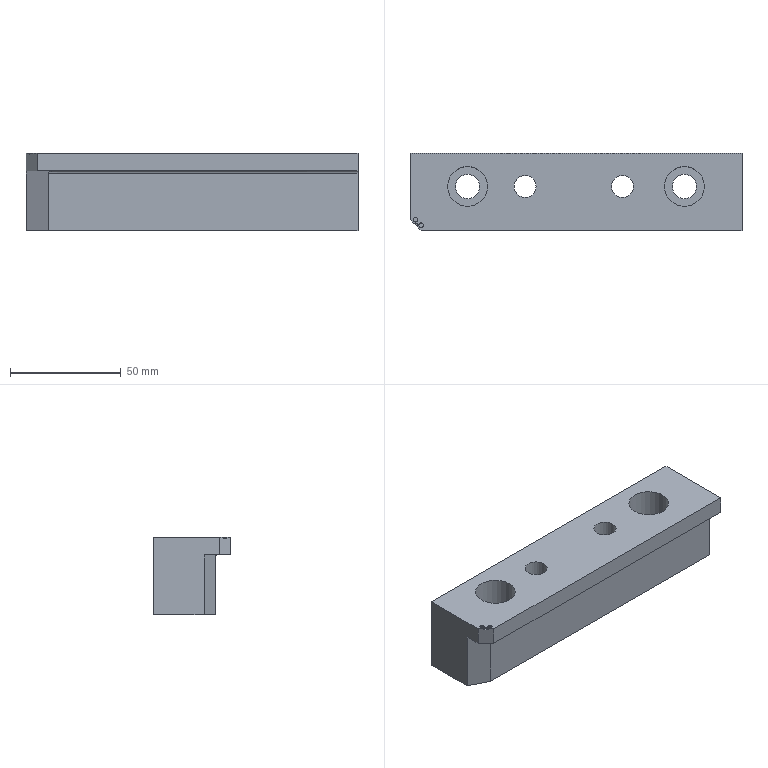Part | NX | features DIE-2 2 | 1 solid | 25 faces | box 150 x 35 x 35 mm | volume 137394 mm3 | plane 15 | cylinder 10 | commonest cylinder face diameters 2 x4 10 x2 11.007 x2 18 x2
STEP:
#1=CARTESIAN_POINT('',(2244.094,-778.422,858.716));
#2=VERTEX_POINT('',#1);
#3=CARTESIAN_POINT('',(2239.094,-778.422,858.716));
#4=DIRECTION('',(0.,0.,1.));
#5=DIRECTION('',(1.,0.,0.));
#6=AXIS2_PLACEMENT_3D('',#3,#4,#5);
#7=CIRCLE('',#6,5.);
#8=EDGE_CURVE('',#2,#2,#7,.T.);
#9=ORIENTED_EDGE('',*,*,#8,.F.);
#10=EDGE_LOOP('',(#9));
#11=FACE_BOUND('',#10,.T.);
#12=CARTESIAN_POINT('',(2244.094,-778.422,893.716));
#13=VERTEX_POINT('',#12);
#14=CARTESIAN_POINT('',(2239.094,-778.422,893.716));
#15=DIRECTION('',(0.,0.,-1.));
#16=DIRECTION('',(1.,0.,0.));
#17=AXIS2_PLACEMENT_3D('',#14,#15,#16);
#18=CIRCLE('',#17,5.);
#19=EDGE_CURVE('',#13,#13,#18,.T.);
#20=ORIENTED_EDGE('',*,*,#19,.F.);
#21=EDGE_LOOP('',(#20));
#22=FACE_BOUND('',#21,.T.);
#23=CARTESIAN_POINT('',(2239.094,-778.422,890.716));
#24=DIRECTION('',(0.,0.,1.));
#25=DIRECTION('',(-1.,0.,0.));
#26=AXIS2_PLACEMENT_3D('',#23,#24,#25);
#27=CYLINDRICAL_SURFACE('',#26,5.);
#28=ADVANCED_FACE('',(#11,#22),#27,.F.);
#29=CARTESIAN_POINT('',(2276.094,-778.422,877.716));
#30=VERTEX_POINT('',#29);
#31=CARTESIAN_POINT('',(2267.094,-778.422,877.716));
#32=DIRECTION('',(0.,0.,-1.));
#33=DIRECTION('',(1.,0.,0.));
#34=AXIS2_PLACEMENT_3D('',#31,#32,#33);
#35=CIRCLE('',#34,9.);
#36=EDGE_CURVE('',#30,#30,#35,.T.);
#37=ORIENTED_EDGE('',*,*,#36,.T.);
#38=EDGE_LOOP('',(#37));
#39=FACE_BOUND('',#38,.T.);
#40=CARTESIAN_POINT('',(2276.094,-778.422,893.716));
#41=VERTEX_POINT('',#40);
#42=CARTESIAN_POINT('',(2267.094,-778.422,893.716));
#43=DIRECTION('',(0.,0.,-1.));
#44=DIRECTION('',(1.,0.,0.));
#45=AXIS2_PLACEMENT_3D('',#42,#43,#44);
#46=CIRCLE('',#45,9.);
#47=EDGE_CURVE('',#41,#41,#46,.T.);
#48=ORIENTED_EDGE('',*,*,#47,.F.);
#49=EDGE_LOOP('',(#48));
#50=FACE_BOUND('',#49,.T.);
#51=CARTESIAN_POINT('',(2267.094,-778.422,884.216));
#52=DIRECTION('',(0.,0.,-1.));
#53=DIRECTION('',(-1.,0.,0.));
#54=AXIS2_PLACEMENT_3D('',#51,#52,#53);
#55=CYLINDRICAL_SURFACE('',#54,9.);
#56=ADVANCED_FACE('',(#39,#50),#55,.F.);
#57=CARTESIAN_POINT('',(2178.094,-778.422,877.716));
#58=VERTEX_POINT('',#57);
#59=CARTESIAN_POINT('',(2169.094,-778.422,877.716));
#60=DIRECTION('',(0.,0.,-1.));
#61=DIRECTION('',(1.,0.,0.));
#62=AXIS2_PLACEMENT_3D('',#59,#60,#61);
#63=CIRCLE('',#62,9.);
#64=EDGE_CURVE('',#58,#58,#63,.T.);
#65=ORIENTED_EDGE('',*,*,#64,.T.);
#66=EDGE_LOOP('',(#65));
#67=FACE_BOUND('',#66,.T.);
#68=CARTESIAN_POINT('',(2178.094,-778.422,893.716));
#69=VERTEX_POINT('',#68);
#70=CARTESIAN_POINT('',(2169.094,-778.422,893.716));
#71=DIRECTION('',(0.,0.,-1.));
#72=DIRECTION('',(1.,0.,0.));
#73=AXIS2_PLACEMENT_3D('',#70,#71,#72);
#74=CIRCLE('',#73,9.);
#75=EDGE_CURVE('',#69,#69,#74,.T.);
#76=ORIENTED_EDGE('',*,*,#75,.F.);
#77=EDGE_LOOP('',(#76));
#78=FACE_BOUND('',#77,.T.);
#79=CARTESIAN_POINT('',(2169.094,-778.422,884.216));
#80=DIRECTION('',(0.,0.,-1.));
#81=DIRECTION('',(-1.,0.,0.));
#82=AXIS2_PLACEMENT_3D('',#79,#80,#81);
#83=CYLINDRICAL_SURFACE('',#82,9.);
#84=ADVANCED_FACE('',(#67,#78),#83,.F.);
#85=CARTESIAN_POINT('',(2200.094,-778.422,858.716));
#86=VERTEX_POINT('',#85);
#87=CARTESIAN_POINT('',(2195.094,-778.422,858.716));
#88=DIRECTION('',(0.,0.,-1.));
#89=DIRECTION('',(1.,0.,0.));
#90=AXIS2_PLACEMENT_3D('',#87,#88,#89);
#91=CIRCLE('',#90,5.);
#92=EDGE_CURVE('',#86,#86,#91,.T.);
#93=ORIENTED_EDGE('',*,*,#92,.T.);
#94=EDGE_LOOP('',(#93));
#95=FACE_BOUND('',#94,.T.);
#96=CARTESIAN_POINT('',(2200.094,-778.422,893.716));
#97=VERTEX_POINT('',#96);
#98=CARTESIAN_POINT('',(2195.094,-778.422,893.716));
#99=DIRECTION('',(0.,0.,-1.));
#100=DIRECTION('',(1.,0.,0.));
#101=AXIS2_PLACEMENT_3D('',#98,#99,#100);
#102=CIRCLE('',#101,5.);
#103=EDGE_CURVE('',#97,#97,#102,.T.);
#104=ORIENTED_EDGE('',*,*,#103,.F.);
#105=EDGE_LOOP('',(#104));
#106=FACE_BOUND('',#105,.T.);
#107=CARTESIAN_POINT('',(2195.094,-778.422,890.716));
#108=DIRECTION('',(0.,0.,1.));
#109=DIRECTION('',(-1.,0.,0.));
#110=AXIS2_PLACEMENT_3D('',#107,#108,#109);
#111=CYLINDRICAL_SURFACE('',#110,5.);
#112=ADVANCED_FACE('',(#95,#106),#111,.F.);
#113=CARTESIAN_POINT('',(2293.094,-763.422,858.716));
#114=VERTEX_POINT('',#113);
#115=CARTESIAN_POINT('',(2293.094,-791.422,858.716));
#116=VERTEX_POINT('',#115);
#117=CARTESIAN_POINT('',(2293.094,-797.422,858.716));
#118=DIRECTION('',(0.,-1.,0.));
#119=VECTOR('',#118,1000.);
#120=LINE('',#117,#119);
#121=EDGE_CURVE('',#114,#116,#120,.T.);
#122=ORIENTED_EDGE('',*,*,#121,.F.);
#123=CARTESIAN_POINT('',(2293.094,-763.422,893.716));
#124=VERTEX_POINT('',#123);
#125=CARTESIAN_POINT('',(2293.094,-763.422,890.716));
#126=DIRECTION('',(0.,0.,-1.));
#127=VECTOR('',#126,1000.);
#128=LINE('',#125,#127);
#129=EDGE_CURVE('',#124,#114,#128,.T.);
#130=ORIENTED_EDGE('',*,*,#129,.F.);
#131=CARTESIAN_POINT('',(2293.094,-798.422,893.716));
#132=VERTEX_POINT('',#131);
#133=CARTESIAN_POINT('',(2293.094,-763.422,893.716));
#134=DIRECTION('',(0.,-1.,0.));
#135=VECTOR('',#134,1000.);
#136=LINE('',#133,#135);
#137=EDGE_CURVE('',#124,#132,#136,.T.);
#138=ORIENTED_EDGE('',*,*,#137,.T.);
#139=CARTESIAN_POINT('',(2293.094,-798.422,885.716));
#140=VERTEX_POINT('',#139);
#141=CARTESIAN_POINT('',(2293.094,-798.422,893.716));
#142=DIRECTION('',(0.,0.,-1.));
#143=VECTOR('',#142,1000.);
#144=LINE('',#141,#143);
#145=EDGE_CURVE('',#132,#140,#144,.T.);
#146=ORIENTED_EDGE('',*,*,#145,.T.);
#147=CARTESIAN_POINT('',(2293.094,-792.422,885.716));
#148=VERTEX_POINT('',#147);
#149=CARTESIAN_POINT('',(2293.094,-797.422,885.716));
#150=DIRECTION('',(0.,-1.,0.));
#151=VECTOR('',#150,1000.);
#152=LINE('',#149,#151);
#153=EDGE_CURVE('',#148,#140,#152,.T.);
#154=ORIENTED_EDGE('',*,*,#153,.F.);
#155=CARTESIAN_POINT('',(2293.094,-791.422,884.716));
#156=VERTEX_POINT('',#155);
#157=CARTESIAN_POINT('',(2293.094,-792.422,884.716));
#158=DIRECTION('',(-1.,0.,0.));
#159=DIRECTION('',(0.,0.,-1.));
#160=AXIS2_PLACEMENT_3D('',#157,#158,#159);
#161=CIRCLE('',#160,1.);
#162=EDGE_CURVE('',#148,#156,#161,.T.);
#163=ORIENTED_EDGE('',*,*,#162,.T.);
#164=CARTESIAN_POINT('',(2293.094,-791.422,890.716));
#165=DIRECTION('',(0.,0.,-1.));
#166=VECTOR('',#165,1000.);
#167=LINE('',#164,#166);
#168=EDGE_CURVE('',#156,#116,#167,.T.);
#169=ORIENTED_EDGE('',*,*,#168,.T.);
#170=EDGE_LOOP('',(#122,#130,#138,#146,#154,#163,#169));
#171=FACE_BOUND('',#170,.T.);
#172=CARTESIAN_POINT('',(2293.094,-797.422,890.716));
#173=DIRECTION('',(1.,0.,0.));
#174=DIRECTION('',(0.,0.,1.));
#175=AXIS2_PLACEMENT_3D('',#172,#173,#174);
#176=PLANE('',#175);
#177=ADVANCED_FACE('',(#171),#176,.T.);
#178=CARTESIAN_POINT('',(2143.094,-763.422,858.716));
#179=VERTEX_POINT('',#178);
#180=CARTESIAN_POINT('',(2293.094,-763.422,858.716));
#181=DIRECTION('',(1.,0.,0.));
#182=VECTOR('',#181,1000.);
#183=LINE('',#180,#182);
#184=EDGE_CURVE('',#179,#114,#183,.T.);
#185=ORIENTED_EDGE('',*,*,#184,.F.);
#186=CARTESIAN_POINT('',(2143.094,-763.422,893.716));
#187=VERTEX_POINT('',#186);
#188=CARTESIAN_POINT('',(2143.094,-763.422,890.716));
#189=DIRECTION('',(0.,0.,1.));
#190=VECTOR('',#189,1000.);
#191=LINE('',#188,#190);
#192=EDGE_CURVE('',#187,#179,#191,.F.);
#193=ORIENTED_EDGE('',*,*,#192,.F.);
#194=CARTESIAN_POINT('',(2118.094,-763.422,893.716));
#195=DIRECTION('',(1.,0.,0.));
#196=VECTOR('',#195,1000.);
#197=LINE('',#194,#196);
#198=EDGE_CURVE('',#187,#124,#197,.T.);
#199=ORIENTED_EDGE('',*,*,#198,.T.);
#200=ORIENTED_EDGE('',*,*,#129,.T.);
#201=EDGE_LOOP('',(#185,#193,#199,#200));
#202=FACE_BOUND('',#201,.T.);
#203=CARTESIAN_POINT('',(2293.094,-763.422,890.716));
#204=DIRECTION('',(0.,1.,0.));
#205=DIRECTION('',(0.,0.,-1.));
#206=AXIS2_PLACEMENT_3D('',#203,#204,#205);
#207=PLANE('',#206);
#208=ADVANCED_FACE('',(#202),#207,.T.);
#209=CARTESIAN_POINT('',(2143.094,-786.422,858.716));
#210=VERTEX_POINT('',#209);
#211=CARTESIAN_POINT('',(2143.094,-810.322,858.716));
#212=DIRECTION('',(0.,-1.,0.));
#213=VECTOR('',#212,1000.);
#214=LINE('',#211,#213);
#215=EDGE_CURVE('',#179,#210,#214,.T.);
#216=ORIENTED_EDGE('',*,*,#215,.T.);
#217=CARTESIAN_POINT('',(2143.094,-786.422,885.716));
#218=VERTEX_POINT('',#217);
#219=CARTESIAN_POINT('',(2143.094,-786.422,882.716));
#220=DIRECTION('',(0.,0.,1.));
#221=VECTOR('',#220,1000.);
#222=LINE('',#219,#221);
#223=EDGE_CURVE('',#210,#218,#222,.T.);
#224=ORIENTED_EDGE('',*,*,#223,.T.);
#225=CARTESIAN_POINT('',(2143.094,-793.422,885.716));
#226=VERTEX_POINT('',#225);
#227=CARTESIAN_POINT('',(2143.094,-768.422,885.716));
#228=DIRECTION('',(0.,-1.,0.));
#229=VECTOR('',#228,1000.);
#230=LINE('',#227,#229);
#231=EDGE_CURVE('',#218,#226,#230,.T.);
#232=ORIENTED_EDGE('',*,*,#231,.T.);
#233=CARTESIAN_POINT('',(2143.094,-793.422,893.716));
#234=VERTEX_POINT('',#233);
#235=CARTESIAN_POINT('',(2143.094,-793.422,893.716));
#236=DIRECTION('',(0.,0.,1.));
#237=VECTOR('',#236,1000.);
#238=LINE('',#235,#237);
#239=EDGE_CURVE('',#226,#234,#238,.T.);
#240=ORIENTED_EDGE('',*,*,#239,.T.);
#241=CARTESIAN_POINT('',(2143.094,-792.422,893.716));
#242=DIRECTION('',(0.,1.,0.));
#243=VECTOR('',#242,1000.);
#244=LINE('',#241,#243);
#245=EDGE_CURVE('',#234,#187,#244,.T.);
#246=ORIENTED_EDGE('',*,*,#245,.T.);
#247=ORIENTED_EDGE('',*,*,#192,.T.);
#248=EDGE_LOOP('',(#216,#224,#232,#240,#246,#247));
#249=FACE_BOUND('',#248,.T.);
#250=CARTESIAN_POINT('',(2143.094,-768.422,890.716));
#251=DIRECTION('',(-1.,0.,0.));
#252=DIRECTION('',(0.,0.,-1.));
#253=AXIS2_PLACEMENT_3D('',#250,#251,#252);
#254=PLANE('',#253);
#255=ADVANCED_FACE('',(#249),#254,.T.);
#256=CARTESIAN_POINT('',(2272.597,-778.422,858.716));
#257=VERTEX_POINT('',#256);
#258=CARTESIAN_POINT('',(2267.094,-778.422,858.716));
#259=DIRECTION('',(0.,0.,1.));
#260=DIRECTION('',(1.,0.,0.));
#261=AXIS2_PLACEMENT_3D('',#258,#259,#260);
#262=CIRCLE('',#261,5.503);
#263=EDGE_CURVE('',#257,#257,#262,.T.);
#264=ORIENTED_EDGE('',*,*,#263,.F.);
#265=EDGE_LOOP('',(#264));
#266=FACE_BOUND('',#265,.T.);
#267=CARTESIAN_POINT('',(2261.59,-778.422,877.716));
#268=VERTEX_POINT('',#267);
#269=CARTESIAN_POINT('',(2267.094,-778.422,877.716));
#270=DIRECTION('',(0.,0.,-1.));
#271=DIRECTION('',(-1.,0.,0.));
#272=AXIS2_PLACEMENT_3D('',#269,#270,#271);
#273=CIRCLE('',#272,5.503);
#274=EDGE_CURVE('',#268,#268,#273,.T.);
#275=ORIENTED_EDGE('',*,*,#274,.F.);
#276=EDGE_LOOP('',(#275));
#277=FACE_BOUND('',#276,.T.);
#278=CARTESIAN_POINT('',(2267.094,-778.422,890.716));
#279=DIRECTION('',(0.,0.,1.));
#280=DIRECTION('',(-1.,0.,0.));
#281=AXIS2_PLACEMENT_3D('',#278,#279,#280);
#282=CYLINDRICAL_SURFACE('',#281,5.503);
#283=ADVANCED_FACE('',(#266,#277),#282,.F.);
#284=ORIENTED_EDGE('',*,*,#274,.T.);
#285=EDGE_LOOP('',(#284));
#286=FACE_BOUND('',#285,.T.);
#287=ORIENTED_EDGE('',*,*,#36,.F.);
#288=EDGE_LOOP('',(#287));
#289=FACE_BOUND('',#288,.T.);
#290=CARTESIAN_POINT('',(2267.094,-778.422,877.716));
#291=DIRECTION('',(0.,0.,-1.));
#292=DIRECTION('',(1.,0.,0.));
#293=AXIS2_PLACEMENT_3D('',#290,#291,#292);
#294=PLANE('',#293);
#295=ADVANCED_FACE('',(#286,#289),#294,.F.);
#296=CARTESIAN_POINT('',(2174.597,-778.422,858.716));
#297=VERTEX_POINT('',#296);
#298=CARTESIAN_POINT('',(2169.094,-778.422,858.716));
#299=DIRECTION('',(0.,0.,1.));
#300=DIRECTION('',(1.,0.,0.));
#301=AXIS2_PLACEMENT_3D('',#298,#299,#300);
#302=CIRCLE('',#301,5.503);
#303=EDGE_CURVE('',#297,#297,#302,.F.);
#304=ORIENTED_EDGE('',*,*,#303,.T.);
#305=EDGE_LOOP('',(#304));
#306=FACE_BOUND('',#305,.T.);
#307=CARTESIAN_POINT('',(2163.59,-778.422,877.716));
#308=VERTEX_POINT('',#307);
#309=CARTESIAN_POINT('',(2169.094,-778.422,877.716));
#310=DIRECTION('',(0.,0.,-1.));
#311=DIRECTION('',(-1.,0.,0.));
#312=AXIS2_PLACEMENT_3D('',#309,#310,#311);
#313=CIRCLE('',#312,5.503);
#314=EDGE_CURVE('',#308,#308,#313,.T.);
#315=ORIENTED_EDGE('',*,*,#314,.F.);
#316=EDGE_LOOP('',(#315));
#317=FACE_BOUND('',#316,.T.);
#318=CARTESIAN_POINT('',(2169.094,-778.422,890.716));
#319=DIRECTION('',(0.,0.,1.));
#320=DIRECTION('',(-1.,0.,0.));
#321=AXIS2_PLACEMENT_3D('',#318,#319,#320);
#322=CYLINDRICAL_SURFACE('',#321,5.503);
#323=ADVANCED_FACE('',(#306,#317),#322,.F.);
#324=ORIENTED_EDGE('',*,*,#314,.T.);
#325=EDGE_LOOP('',(#324));
#326=FACE_BOUND('',#325,.T.);
#327=ORIENTED_EDGE('',*,*,#64,.F.);
#328=EDGE_LOOP('',(#327));
#329=FACE_BOUND('',#328,.T.);
#330=CARTESIAN_POINT('',(2169.094,-778.422,877.716));
#331=DIRECTION('',(0.,0.,-1.));
#332=DIRECTION('',(1.,0.,0.));
#333=AXIS2_PLACEMENT_3D('',#330,#331,#332);
#334=PLANE('',#333);
#335=ADVANCED_FACE('',(#326,#329),#334,.F.);
#336=CARTESIAN_POINT('',(2153.094,-791.422,884.716));
#337=VERTEX_POINT('',#336);
#338=CARTESIAN_POINT('',(2153.094,-791.422,858.716));
#339=VERTEX_POINT('',#338);
#340=CARTESIAN_POINT('',(2153.094,-791.422,844.716));
#341=DIRECTION('',(0.,0.,-1.));
#342=VECTOR('',#341,1000.);
#343=LINE('',#340,#342);
#344=EDGE_CURVE('',#337,#339,#343,.T.);
#345=ORIENTED_EDGE('',*,*,#344,.T.);
#346=CARTESIAN_POINT('',(2113.094,-791.422,858.716));
#347=DIRECTION('',(1.,0.,0.));
#348=VECTOR('',#347,1000.);
#349=LINE('',#346,#348);
#350=EDGE_CURVE('',#339,#116,#349,.T.);
#351=ORIENTED_EDGE('',*,*,#350,.T.);
#352=ORIENTED_EDGE('',*,*,#168,.F.);
#353=CARTESIAN_POINT('',(2123.094,-791.422,884.716));
#354=DIRECTION('',(-1.,0.,0.));
#355=VECTOR('',#354,1000.);
#356=LINE('',#353,#355);
#357=EDGE_CURVE('',#156,#337,#356,.T.);
#358=ORIENTED_EDGE('',*,*,#357,.T.);
#359=EDGE_LOOP('',(#345,#351,#352,#358));
#360=FACE_BOUND('',#359,.T.);
#361=CARTESIAN_POINT('',(2113.094,-791.422,890.716));
#362=DIRECTION('',(0.,1.,0.));
#363=DIRECTION('',(0.,0.,-1.));
#364=AXIS2_PLACEMENT_3D('',#361,#362,#363);
#365=PLANE('',#364);
#366=ADVANCED_FACE('',(#360),#365,.F.);
#367=ORIENTED_EDGE('',*,*,#231,.F.);
#368=CARTESIAN_POINT('',(2155.094,-792.422,885.716));
#369=VERTEX_POINT('',#368);
#370=CARTESIAN_POINT('',(2212.694,-821.222,885.716));
#371=DIRECTION('',(0.8944,-0.4472,0.));
#372=VECTOR('',#371,1000.);
#373=LINE('',#370,#372);
#374=EDGE_CURVE('',#218,#369,#373,.T.);
#375=ORIENTED_EDGE('',*,*,#374,.T.);
#376=CARTESIAN_POINT('',(2293.094,-792.422,885.716));
#377=DIRECTION('',(1.,0.,0.));
#378=VECTOR('',#377,1000.);
#379=LINE('',#376,#378);
#380=EDGE_CURVE('',#369,#148,#379,.T.);
#381=ORIENTED_EDGE('',*,*,#380,.T.);
#382=ORIENTED_EDGE('',*,*,#153,.T.);
#383=CARTESIAN_POINT('',(2148.094,-798.422,885.716));
#384=VERTEX_POINT('',#383);
#385=CARTESIAN_POINT('',(2203.094,-798.422,885.716));
#386=DIRECTION('',(1.,0.,0.));
#387=VECTOR('',#386,1000.);
#388=LINE('',#385,#387);
#389=EDGE_CURVE('',#384,#140,#388,.T.);
#390=ORIENTED_EDGE('',*,*,#389,.F.);
#391=CARTESIAN_POINT('',(2148.094,-798.422,885.716));
#392=DIRECTION('',(-0.7071,0.7071,0.));
#393=VECTOR('',#392,1000.);
#394=LINE('',#391,#393);
#395=EDGE_CURVE('',#384,#226,#394,.T.);
#396=ORIENTED_EDGE('',*,*,#395,.T.);
#397=EDGE_LOOP('',(#367,#375,#381,#382,#390,#396));
#398=FACE_BOUND('',#397,.T.);
#399=CARTESIAN_POINT('',(2203.094,-780.422,885.716));
#400=DIRECTION('',(0.,0.,1.));
#401=DIRECTION('',(-1.,0.,0.));
#402=AXIS2_PLACEMENT_3D('',#399,#400,#401);
#403=PLANE('',#402);
#404=ADVANCED_FACE('',(#398),#403,.F.);
#405=CARTESIAN_POINT('',(2146.594,-793.422,893.716));
#406=VERTEX_POINT('',#405);
#407=CARTESIAN_POINT('',(2145.594,-793.422,893.716));
#408=DIRECTION('',(0.,0.,1.));
#409=DIRECTION('',(1.,0.,0.));
#410=AXIS2_PLACEMENT_3D('',#407,#408,#409);
#411=CIRCLE('',#410,1.);
#412=EDGE_CURVE('',#406,#406,#411,.T.);
#413=ORIENTED_EDGE('',*,*,#412,.F.);
#414=EDGE_LOOP('',(#413));
#415=FACE_BOUND('',#414,.T.);
#416=CARTESIAN_POINT('',(2149.094,-795.922,893.716));
#417=VERTEX_POINT('',#416);
#418=CARTESIAN_POINT('',(2148.094,-795.922,893.716));
#419=DIRECTION('',(0.,0.,1.));
#420=DIRECTION('',(1.,0.,0.));
#421=AXIS2_PLACEMENT_3D('',#418,#419,#420);
#422=CIRCLE('',#421,1.);
#423=EDGE_CURVE('',#417,#417,#422,.T.);
#424=ORIENTED_EDGE('',*,*,#423,.F.);
#425=EDGE_LOOP('',(#424));
#426=FACE_BOUND('',#425,.T.);
#427=CARTESIAN_POINT('',(2146.301,-796.629,893.716));
#428=VERTEX_POINT('',#427);
#429=CARTESIAN_POINT('',(2144.887,-795.215,893.716));
#430=VERTEX_POINT('',#429);
#431=CARTESIAN_POINT('',(2145.594,-795.922,893.716));
#432=DIRECTION('',(0.,0.,1.));
#433=DIRECTION('',(1.,0.,0.));
#434=AXIS2_PLACEMENT_3D('',#431,#432,#433);
#435=CIRCLE('',#434,1.);
#436=EDGE_CURVE('',#428,#430,#435,.T.);
#437=ORIENTED_EDGE('',*,*,#436,.F.);
#438=CARTESIAN_POINT('',(2148.094,-798.422,893.716));
#439=VERTEX_POINT('',#438);
#440=CARTESIAN_POINT('',(2182.27,-832.598,893.716));
#441=DIRECTION('',(0.7071,-0.7071,0.));
#442=VECTOR('',#441,1000.);
#443=LINE('',#440,#442);
#444=EDGE_CURVE('',#428,#439,#443,.T.);
#445=ORIENTED_EDGE('',*,*,#444,.T.);
#446=CARTESIAN_POINT('',(2120.235,-798.422,893.716));
#447=DIRECTION('',(-1.,0.,0.));
#448=VECTOR('',#447,1000.);
#449=LINE('',#446,#448);
#450=EDGE_CURVE('',#132,#439,#449,.T.);
#451=ORIENTED_EDGE('',*,*,#450,.F.);
#452=ORIENTED_EDGE('',*,*,#137,.F.);
#453=ORIENTED_EDGE('',*,*,#198,.F.);
#454=ORIENTED_EDGE('',*,*,#245,.F.);
#455=CARTESIAN_POINT('',(2182.27,-832.598,893.716));
#456=DIRECTION('',(0.7071,-0.7071,0.));
#457=VECTOR('',#456,1000.);
#458=LINE('',#455,#457);
#459=EDGE_CURVE('',#234,#430,#458,.T.);
#460=ORIENTED_EDGE('',*,*,#459,.T.);
#461=EDGE_LOOP('',(#437,#445,#451,#452,#453,#454,#460));
#462=FACE_BOUND('',#461,.T.);
#463=ORIENTED_EDGE('',*,*,#19,.T.);
#464=EDGE_LOOP('',(#463));
#465=FACE_BOUND('',#464,.T.);
#466=ORIENTED_EDGE('',*,*,#47,.T.);
#467=EDGE_LOOP('',(#466));
#468=FACE_BOUND('',#467,.T.);
#469=ORIENTED_EDGE('',*,*,#75,.T.);
#470=EDGE_LOOP('',(#469));
#471=FACE_BOUND('',#470,.T.);
#472=ORIENTED_EDGE('',*,*,#103,.T.);
#473=EDGE_LOOP('',(#472));
#474=FACE_BOUND('',#473,.T.);
#475=CARTESIAN_POINT('',(2204.475,-780.392,893.716));
#476=DIRECTION('',(0.,0.,1.));
#477=DIRECTION('',(-1.,0.,0.));
#478=AXIS2_PLACEMENT_3D('',#475,#476,#477);
#479=PLANE('',#478);
#480=ADVANCED_FACE('',(#415,#426,#462,#465,#468,#471,#474),#479,.T.);
#481=ORIENTED_EDGE('',*,*,#450,.T.);
#482=CARTESIAN_POINT('',(2148.094,-798.422,893.716));
#483=DIRECTION('',(0.,0.,-1.));
#484=VECTOR('',#483,1000.);
#485=LINE('',#482,#484);
#486=EDGE_CURVE('',#439,#384,#485,.T.);
#487=ORIENTED_EDGE('',*,*,#486,.T.);
#488=ORIENTED_EDGE('',*,*,#389,.T.);
#489=ORIENTED_EDGE('',*,*,#145,.F.);
#490=EDGE_LOOP('',(#481,#487,#488,#489));
#491=FACE_BOUND('',#490,.T.);
#492=CARTESIAN_POINT('',(2120.235,-798.422,893.716));
#493=DIRECTION('',(0.,-1.,0.));
#494=DIRECTION('',(0.,0.,1.));
#495=AXIS2_PLACEMENT_3D('',#492,#493,#494);
#496=PLANE('',#495);
#497=ADVANCED_FACE('',(#491),#496,.T.);
#498=CARTESIAN_POINT('',(2153.094,-791.422,858.716));
#499=DIRECTION('',(-0.8944,0.4472,0.));
#500=VECTOR('',#499,1000.);
#501=LINE('',#498,#500);
#502=EDGE_CURVE('',#339,#210,#501,.T.);
#503=ORIENTED_EDGE('',*,*,#502,.F.);
#504=ORIENTED_EDGE('',*,*,#344,.F.);
#505=CARTESIAN_POINT('',(2155.094,-792.422,884.716));
#506=DIRECTION('',(0.4472,0.8944,0.));
#507=DIRECTION('',(-0.8944,0.4472,0.));
#508=AXIS2_PLACEMENT_3D('',#505,#506,#507);
#509=ELLIPSE('',#508,2.236,1.);
#510=EDGE_CURVE('',#337,#369,#509,.T.);
#511=ORIENTED_EDGE('',*,*,#510,.T.);
#512=ORIENTED_EDGE('',*,*,#374,.F.);
#513=ORIENTED_EDGE('',*,*,#223,.F.);
#514=EDGE_LOOP('',(#503,#504,#511,#512,#513));
#515=FACE_BOUND('',#514,.T.);
#516=CARTESIAN_POINT('',(2153.094,-791.422,890.716));
#517=DIRECTION('',(-0.4472,-0.8944,0.));
#518=DIRECTION('',(0.,0.,-1.));
#519=AXIS2_PLACEMENT_3D('',#516,#517,#518);
#520=PLANE('',#519);
#521=ADVANCED_FACE('',(#515),#520,.T.);
#522=CARTESIAN_POINT('',(2144.887,-795.215,893.216));
#523=VERTEX_POINT('',#522);
#524=CARTESIAN_POINT('',(2146.301,-796.629,893.216));
#525=VERTEX_POINT('',#524);
#526=CARTESIAN_POINT('',(2148.094,-798.422,893.216));
#527=DIRECTION('',(0.7071,-0.7071,0.));
#528=VECTOR('',#527,1000.);
#529=LINE('',#526,#528);
#530=EDGE_CURVE('',#523,#525,#529,.T.);
#531=ORIENTED_EDGE('',*,*,#530,.F.);
#532=CARTESIAN_POINT('',(2144.887,-795.215,893.216));
#533=DIRECTION('',(0.,0.,1.));
#534=VECTOR('',#533,1000.);
#535=LINE('',#532,#534);
#536=EDGE_CURVE('',#523,#430,#535,.T.);
#537=ORIENTED_EDGE('',*,*,#536,.T.);
#538=ORIENTED_EDGE('',*,*,#459,.F.);
#539=ORIENTED_EDGE('',*,*,#239,.F.);
#540=ORIENTED_EDGE('',*,*,#395,.F.);
#541=ORIENTED_EDGE('',*,*,#486,.F.);
#542=ORIENTED_EDGE('',*,*,#444,.F.);
#543=CARTESIAN_POINT('',(2146.301,-796.629,893.216));
#544=DIRECTION('',(0.,0.,1.));
#545=VECTOR('',#544,1000.);
#546=LINE('',#543,#545);
#547=EDGE_CURVE('',#428,#525,#546,.F.);
#548=ORIENTED_EDGE('',*,*,#547,.T.);
#549=EDGE_LOOP('',(#531,#537,#538,#539,#540,#541,#542,#548));
#550=FACE_BOUND('',#549,.T.);
#551=CARTESIAN_POINT('',(2148.094,-798.422,893.716));
#552=DIRECTION('',(0.7071,0.7071,0.));
#553=DIRECTION('',(0.,0.,1.));
#554=AXIS2_PLACEMENT_3D('',#551,#552,#553);
#555=PLANE('',#554);
#556=ADVANCED_FACE('',(#550),#555,.F.);
#557=ORIENTED_EDGE('',*,*,#162,.F.);
#558=ORIENTED_EDGE('',*,*,#380,.F.);
#559=ORIENTED_EDGE('',*,*,#510,.F.);
#560=ORIENTED_EDGE('',*,*,#357,.F.);
#561=EDGE_LOOP('',(#557,#558,#559,#560));
#562=FACE_BOUND('',#561,.T.);
#563=CARTESIAN_POINT('',(2203.094,-792.422,884.716));
#564=DIRECTION('',(-1.,0.,0.));
#565=DIRECTION('',(0.,0.,-1.));
#566=AXIS2_PLACEMENT_3D('',#563,#564,#565);
#567=CYLINDRICAL_SURFACE('',#566,1.);
#568=ADVANCED_FACE('',(#562),#567,.F.);
#569=ORIENTED_EDGE('',*,*,#92,.F.);
#570=EDGE_LOOP('',(#569));
#571=FACE_BOUND('',#570,.T.);
#572=ORIENTED_EDGE('',*,*,#303,.F.);
#573=EDGE_LOOP('',(#572));
#574=FACE_BOUND('',#573,.T.);
#575=ORIENTED_EDGE('',*,*,#121,.T.);
#576=ORIENTED_EDGE('',*,*,#350,.F.);
#577=ORIENTED_EDGE('',*,*,#502,.T.);
#578=ORIENTED_EDGE('',*,*,#215,.F.);
#579=ORIENTED_EDGE('',*,*,#184,.T.);
#580=EDGE_LOOP('',(#575,#576,#577,#578,#579));
#581=FACE_BOUND('',#580,.T.);
#582=ORIENTED_EDGE('',*,*,#263,.T.);
#583=EDGE_LOOP('',(#582));
#584=FACE_BOUND('',#583,.T.);
#585=ORIENTED_EDGE('',*,*,#8,.T.);
#586=EDGE_LOOP('',(#585));
#587=FACE_BOUND('',#586,.T.);
#588=CARTESIAN_POINT('',(2203.862,-810.322,858.716));
#589=DIRECTION('',(0.,0.,1.));
#590=DIRECTION('',(-1.,0.,0.));
#591=AXIS2_PLACEMENT_3D('',#588,#589,#590);
#592=PLANE('',#591);
#593=ADVANCED_FACE('',(#571,#574,#581,#584,#587),#592,.F.);
#594=CARTESIAN_POINT('',(2145.594,-795.922,893.216));
#595=DIRECTION('',(0.,0.,1.));
#596=DIRECTION('',(1.,0.,0.));
#597=AXIS2_PLACEMENT_3D('',#594,#595,#596);
#598=CIRCLE('',#597,1.);
#599=EDGE_CURVE('',#523,#525,#598,.F.);
#600=ORIENTED_EDGE('',*,*,#599,.T.);
#601=ORIENTED_EDGE('',*,*,#547,.F.);
#602=ORIENTED_EDGE('',*,*,#436,.T.);
#603=ORIENTED_EDGE('',*,*,#536,.F.);
#604=EDGE_LOOP('',(#600,#601,#602,#603));
#605=FACE_BOUND('',#604,.T.);
#606=CARTESIAN_POINT('',(2145.594,-795.922,893.216));
#607=DIRECTION('',(0.,0.,1.));
#608=DIRECTION('',(1.,0.,0.));
#609=AXIS2_PLACEMENT_3D('',#606,#607,#608);
#610=CYLINDRICAL_SURFACE('',#609,1.);
#611=ADVANCED_FACE('',(#605),#610,.F.);
#612=ORIENTED_EDGE('',*,*,#530,.T.);
#613=ORIENTED_EDGE('',*,*,#599,.F.);
#614=EDGE_LOOP('',(#612,#613));
#615=FACE_BOUND('',#614,.T.);
#616=CARTESIAN_POINT('',(2145.594,-795.922,893.216));
#617=DIRECTION('',(0.,0.,1.));
#618=DIRECTION('',(1.,0.,0.));
#619=AXIS2_PLACEMENT_3D('',#616,#617,#618);
#620=PLANE('',#619);
#621=ADVANCED_FACE('',(#615),#620,.T.);
#622=CARTESIAN_POINT('',(2149.094,-795.922,893.216));
#623=VERTEX_POINT('',#622);
#624=CARTESIAN_POINT('',(2148.094,-795.922,893.216));
#625=DIRECTION('',(0.,0.,1.));
#626=DIRECTION('',(1.,0.,0.));
#627=AXIS2_PLACEMENT_3D('',#624,#625,#626);
#628=CIRCLE('',#627,1.);
#629=EDGE_CURVE('',#623,#623,#628,.F.);
#630=ORIENTED_EDGE('',*,*,#629,.T.);
#631=EDGE_LOOP('',(#630));
#632=FACE_BOUND('',#631,.T.);
#633=ORIENTED_EDGE('',*,*,#423,.T.);
#634=EDGE_LOOP('',(#633));
#635=FACE_BOUND('',#634,.T.);
#636=CARTESIAN_POINT('',(2148.094,-795.922,893.216));
#637=DIRECTION('',(0.,0.,1.));
#638=DIRECTION('',(1.,0.,0.));
#639=AXIS2_PLACEMENT_3D('',#636,#637,#638);
#640=CYLINDRICAL_SURFACE('',#639,1.);
#641=ADVANCED_FACE('',(#632,#635),#640,.F.);
#642=ORIENTED_EDGE('',*,*,#629,.F.);
#643=EDGE_LOOP('',(#642));
#644=FACE_BOUND('',#643,.T.);
#645=CARTESIAN_POINT('',(2148.094,-795.922,893.216));
#646=DIRECTION('',(0.,0.,1.));
#647=DIRECTION('',(1.,0.,0.));
#648=AXIS2_PLACEMENT_3D('',#645,#646,#647);
#649=PLANE('',#648);
#650=ADVANCED_FACE('',(#644),#649,.T.);
#651=CARTESIAN_POINT('',(2146.594,-793.422,893.216));
#652=VERTEX_POINT('',#651);
#653=CARTESIAN_POINT('',(2145.594,-793.422,893.216));
#654=DIRECTION('',(0.,0.,1.));
#655=DIRECTION('',(1.,0.,0.));
#656=AXIS2_PLACEMENT_3D('',#653,#654,#655);
#657=CIRCLE('',#656,1.);
#658=EDGE_CURVE('',#652,#652,#657,.F.);
#659=ORIENTED_EDGE('',*,*,#658,.T.);
#660=EDGE_LOOP('',(#659));
#661=FACE_BOUND('',#660,.T.);
#662=ORIENTED_EDGE('',*,*,#412,.T.);
#663=EDGE_LOOP('',(#662));
#664=FACE_BOUND('',#663,.T.);
#665=CARTESIAN_POINT('',(2145.594,-793.422,893.216));
#666=DIRECTION('',(0.,0.,1.));
#667=DIRECTION('',(1.,0.,0.));
#668=AXIS2_PLACEMENT_3D('',#665,#666,#667);
#669=CYLINDRICAL_SURFACE('',#668,1.);
#670=ADVANCED_FACE('',(#661,#664),#669,.F.);
#671=ORIENTED_EDGE('',*,*,#658,.F.);
#672=EDGE_LOOP('',(#671));
#673=FACE_BOUND('',#672,.T.);
#674=CARTESIAN_POINT('',(2145.594,-793.422,893.216));
#675=DIRECTION('',(0.,0.,1.));
#676=DIRECTION('',(1.,0.,0.));
#677=AXIS2_PLACEMENT_3D('',#674,#675,#676);
#678=PLANE('',#677);
#679=ADVANCED_FACE('',(#673),#678,.T.);
#680=CLOSED_SHELL('',(#28,#56,#84,#112,#177,#208,#255,#283,#295,#323,#335,#366,#404,#480,#497,#521,#556,#568,#593,#611,#621,#641,#650,#670,#679));
#681=MANIFOLD_SOLID_BREP('',#680);
#682=(LENGTH_UNIT()NAMED_UNIT(*)SI_UNIT(.MILLI.,.METRE.));
#683=UNCERTAINTY_MEASURE_WITH_UNIT(LENGTH_MEASURE(0.00001),#682,'','');
#684=(NAMED_UNIT(*)PLANE_ANGLE_UNIT()SI_UNIT($,.RADIAN.));
#685=(NAMED_UNIT(*)SI_UNIT($,.STERADIAN.)SOLID_ANGLE_UNIT());
#686=(GEOMETRIC_REPRESENTATION_CONTEXT(3)GLOBAL_UNCERTAINTY_ASSIGNED_CONTEXT((#683))GLOBAL_UNIT_ASSIGNED_CONTEXT((#682,#684,#685))REPRESENTATION_CONTEXT('',''));
#687=ADVANCED_BREP_SHAPE_REPRESENTATION('',(#681),#686);